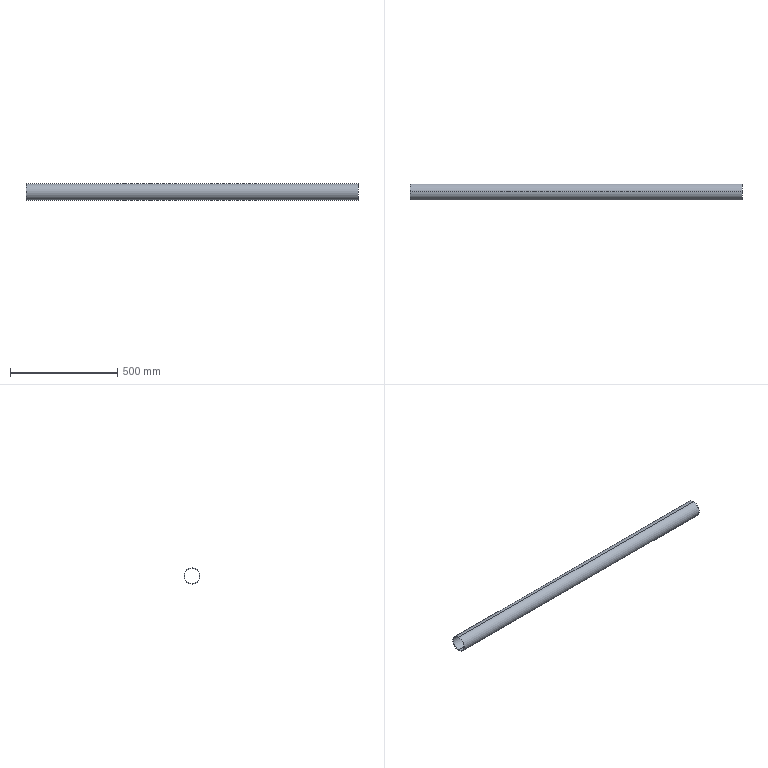Part | STEP file | Microwave Drying Flat Conveyor-CN2500x400-107-102 | 1 solid | 6 faces | box 1550 x 75 x 75 mm | volume 710942 mm3 | cylinder 4 | plane 2 | commonest cylinder face diameters 71 x2 75 x2
STEP:
#1=CARTESIAN_POINT('',(775.,0.,37.5));
#2=VERTEX_POINT('',#1);
#3=CARTESIAN_POINT('',(775.,0.,-37.5));
#4=VERTEX_POINT('',#3);
#5=CARTESIAN_POINT('',(775.,0.,0.));
#6=DIRECTION('',(-1.,0.,0.));
#7=DIRECTION('',(0.,0.,1.));
#8=AXIS2_PLACEMENT_3D('',#5,#6,#7);
#9=CIRCLE('',#8,37.5);
#10=EDGE_CURVE('',#2,#4,#9,.T.);
#11=ORIENTED_EDGE('',*,*,#10,.T.);
#12=CARTESIAN_POINT('',(-775.,0.,-37.5));
#13=VERTEX_POINT('',#12);
#14=CARTESIAN_POINT('',(0.,0.,-37.5));
#15=DIRECTION('',(-1.,0.,0.));
#16=VECTOR('',#15,1000.);
#17=LINE('',#14,#16);
#18=EDGE_CURVE('',#4,#13,#17,.T.);
#19=ORIENTED_EDGE('',*,*,#18,.T.);
#20=CARTESIAN_POINT('',(-775.,0.,37.5));
#21=VERTEX_POINT('',#20);
#22=CARTESIAN_POINT('',(-775.,0.,0.));
#23=DIRECTION('',(-1.,0.,0.));
#24=DIRECTION('',(0.,0.,1.));
#25=AXIS2_PLACEMENT_3D('',#22,#23,#24);
#26=CIRCLE('',#25,37.5);
#27=EDGE_CURVE('',#21,#13,#26,.T.);
#28=ORIENTED_EDGE('',*,*,#27,.F.);
#29=CARTESIAN_POINT('',(0.,0.,37.5));
#30=DIRECTION('',(-1.,0.,0.));
#31=VECTOR('',#30,1000.);
#32=LINE('',#29,#31);
#33=EDGE_CURVE('',#2,#21,#32,.T.);
#34=ORIENTED_EDGE('',*,*,#33,.F.);
#35=EDGE_LOOP('',(#11,#19,#28,#34));
#36=FACE_OUTER_BOUND('',#35,.T.);
#37=CARTESIAN_POINT('',(0.,0.,0.));
#38=DIRECTION('',(-1.,0.,0.));
#39=DIRECTION('',(0.,0.,1.));
#40=AXIS2_PLACEMENT_3D('',#37,#38,#39);
#41=CYLINDRICAL_SURFACE('',#40,37.5);
#42=ADVANCED_FACE('',(#36),#41,.T.);
#43=CARTESIAN_POINT('',(775.,0.,-35.5));
#44=VERTEX_POINT('',#43);
#45=CARTESIAN_POINT('',(775.,0.,35.5));
#46=VERTEX_POINT('',#45);
#47=CARTESIAN_POINT('',(775.,0.,0.));
#48=DIRECTION('',(-1.,0.,0.));
#49=DIRECTION('',(0.,0.,1.));
#50=AXIS2_PLACEMENT_3D('',#47,#48,#49);
#51=CIRCLE('',#50,35.5);
#52=EDGE_CURVE('',#44,#46,#51,.T.);
#53=ORIENTED_EDGE('',*,*,#52,.F.);
#54=CARTESIAN_POINT('',(-775.,0.,-35.5));
#55=VERTEX_POINT('',#54);
#56=CARTESIAN_POINT('',(0.,0.,-35.5));
#57=DIRECTION('',(-1.,0.,0.));
#58=VECTOR('',#57,1000.);
#59=LINE('',#56,#58);
#60=EDGE_CURVE('',#44,#55,#59,.T.);
#61=ORIENTED_EDGE('',*,*,#60,.T.);
#62=CARTESIAN_POINT('',(-775.,0.,35.5));
#63=VERTEX_POINT('',#62);
#64=CARTESIAN_POINT('',(-775.,0.,0.));
#65=DIRECTION('',(-1.,0.,0.));
#66=DIRECTION('',(0.,0.,1.));
#67=AXIS2_PLACEMENT_3D('',#64,#65,#66);
#68=CIRCLE('',#67,35.5);
#69=EDGE_CURVE('',#55,#63,#68,.T.);
#70=ORIENTED_EDGE('',*,*,#69,.T.);
#71=CARTESIAN_POINT('',(0.,0.,35.5));
#72=DIRECTION('',(-1.,0.,0.));
#73=VECTOR('',#72,1000.);
#74=LINE('',#71,#73);
#75=EDGE_CURVE('',#46,#63,#74,.T.);
#76=ORIENTED_EDGE('',*,*,#75,.F.);
#77=EDGE_LOOP('',(#53,#61,#70,#76));
#78=FACE_OUTER_BOUND('',#77,.T.);
#79=CARTESIAN_POINT('',(0.,0.,0.));
#80=DIRECTION('',(-1.,0.,0.));
#81=DIRECTION('',(0.,0.,1.));
#82=AXIS2_PLACEMENT_3D('',#79,#80,#81);
#83=CYLINDRICAL_SURFACE('',#82,35.5);
#84=ADVANCED_FACE('',(#78),#83,.F.);
#85=CARTESIAN_POINT('',(-775.,0.,0.));
#86=DIRECTION('',(-1.,0.,0.));
#87=DIRECTION('',(0.,0.,1.));
#88=AXIS2_PLACEMENT_3D('',#85,#86,#87);
#89=CIRCLE('',#88,35.5);
#90=EDGE_CURVE('',#63,#55,#89,.T.);
#91=ORIENTED_EDGE('',*,*,#90,.F.);
#92=ORIENTED_EDGE('',*,*,#69,.F.);
#93=EDGE_LOOP('',(#91,#92));
#94=FACE_BOUND('',#93,.T.);
#95=ORIENTED_EDGE('',*,*,#27,.T.);
#96=CARTESIAN_POINT('',(-775.,0.,0.));
#97=DIRECTION('',(-1.,0.,0.));
#98=DIRECTION('',(0.,0.,1.));
#99=AXIS2_PLACEMENT_3D('',#96,#97,#98);
#100=CIRCLE('',#99,37.5);
#101=EDGE_CURVE('',#13,#21,#100,.T.);
#102=ORIENTED_EDGE('',*,*,#101,.T.);
#103=EDGE_LOOP('',(#95,#102));
#104=FACE_OUTER_BOUND('',#103,.T.);
#105=CARTESIAN_POINT('',(-775.,37.5,0.));
#106=DIRECTION('',(1.,0.,0.));
#107=DIRECTION('',(0.,0.,-1.));
#108=AXIS2_PLACEMENT_3D('',#105,#106,#107);
#109=PLANE('',#108);
#110=ADVANCED_FACE('',(#94,#104),#109,.F.);
#111=ORIENTED_EDGE('',*,*,#60,.F.);
#112=CARTESIAN_POINT('',(775.,0.,0.));
#113=DIRECTION('',(-1.,0.,0.));
#114=DIRECTION('',(0.,0.,1.));
#115=AXIS2_PLACEMENT_3D('',#112,#113,#114);
#116=CIRCLE('',#115,35.5);
#117=EDGE_CURVE('',#46,#44,#116,.T.);
#118=ORIENTED_EDGE('',*,*,#117,.F.);
#119=ORIENTED_EDGE('',*,*,#75,.T.);
#120=ORIENTED_EDGE('',*,*,#90,.T.);
#121=EDGE_LOOP('',(#111,#118,#119,#120));
#122=FACE_OUTER_BOUND('',#121,.T.);
#123=CARTESIAN_POINT('',(0.,0.,0.));
#124=DIRECTION('',(-1.,0.,0.));
#125=DIRECTION('',(0.,0.,1.));
#126=AXIS2_PLACEMENT_3D('',#123,#124,#125);
#127=CYLINDRICAL_SURFACE('',#126,35.5);
#128=ADVANCED_FACE('',(#122),#127,.F.);
#129=ORIENTED_EDGE('',*,*,#10,.F.);
#130=CARTESIAN_POINT('',(775.,0.,0.));
#131=DIRECTION('',(-1.,0.,0.));
#132=DIRECTION('',(0.,0.,1.));
#133=AXIS2_PLACEMENT_3D('',#130,#131,#132);
#134=CIRCLE('',#133,37.5);
#135=EDGE_CURVE('',#4,#2,#134,.T.);
#136=ORIENTED_EDGE('',*,*,#135,.F.);
#137=EDGE_LOOP('',(#129,#136));
#138=FACE_OUTER_BOUND('',#137,.T.);
#139=ORIENTED_EDGE('',*,*,#117,.T.);
#140=ORIENTED_EDGE('',*,*,#52,.T.);
#141=EDGE_LOOP('',(#139,#140));
#142=FACE_BOUND('',#141,.T.);
#143=CARTESIAN_POINT('',(775.,35.5,0.));
#144=DIRECTION('',(-1.,0.,0.));
#145=DIRECTION('',(0.,0.,1.));
#146=AXIS2_PLACEMENT_3D('',#143,#144,#145);
#147=PLANE('',#146);
#148=ADVANCED_FACE('',(#138,#142),#147,.F.);
#149=ORIENTED_EDGE('',*,*,#18,.F.);
#150=ORIENTED_EDGE('',*,*,#135,.T.);
#151=ORIENTED_EDGE('',*,*,#33,.T.);
#152=ORIENTED_EDGE('',*,*,#101,.F.);
#153=EDGE_LOOP('',(#149,#150,#151,#152));
#154=FACE_OUTER_BOUND('',#153,.T.);
#155=CARTESIAN_POINT('',(0.,0.,0.));
#156=DIRECTION('',(-1.,0.,0.));
#157=DIRECTION('',(0.,0.,1.));
#158=AXIS2_PLACEMENT_3D('',#155,#156,#157);
#159=CYLINDRICAL_SURFACE('',#158,37.5);
#160=ADVANCED_FACE('',(#154),#159,.T.);
#161=CLOSED_SHELL('',(#42,#84,#110,#128,#148,#160));
#162=MANIFOLD_SOLID_BREP('',#161);
#163=CARTESIAN_POINT('',(0.,0.,0.));
#164=DIRECTION('',(0.,0.,1.));
#165=DIRECTION('',(1.,0.,0.));
#166=AXIS2_PLACEMENT_3D('',#163,#164,#165);
#167=(LENGTH_UNIT()NAMED_UNIT(*)SI_UNIT(.MILLI.,.METRE.));
#168=UNCERTAINTY_MEASURE_WITH_UNIT(LENGTH_MEASURE(0.00001),#167,'','');
#169=(NAMED_UNIT(*)PLANE_ANGLE_UNIT()SI_UNIT($,.RADIAN.));
#170=(NAMED_UNIT(*)SI_UNIT($,.STERADIAN.)SOLID_ANGLE_UNIT());
#171=(GEOMETRIC_REPRESENTATION_CONTEXT(3)GLOBAL_UNCERTAINTY_ASSIGNED_CONTEXT((#168))GLOBAL_UNIT_ASSIGNED_CONTEXT((#167,#169,#170))REPRESENTATION_CONTEXT('',''));
#172=ADVANCED_BREP_SHAPE_REPRESENTATION('',(#162,#166),#171);